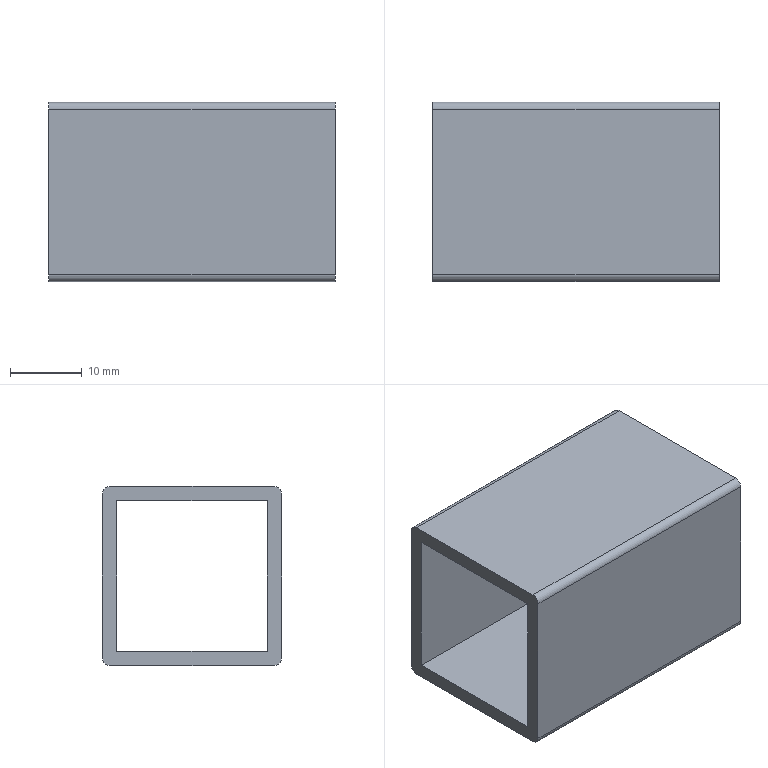Part | SolidWorks | features BreakCorner 1, FlatPattern 1, SMBaseFlange 1, SheetMetal 1 | 1 solid | 14 faces | box 40 x 25 x 25 mm | volume 7326 mm3 | plane 10 | cylinder 4 | commonest cylinder face diameters 2 x4
STEP:
#1=CARTESIAN_POINT('',(-40.,11.5,12.5));
#2=VERTEX_POINT('',#1);
#3=CARTESIAN_POINT('',(-40.,-11.5,12.5));
#4=VERTEX_POINT('',#3);
#5=CARTESIAN_POINT('',(-40.,12.5,12.5));
#6=DIRECTION('',(0.,-1.,0.));
#7=VECTOR('',#6,1000.);
#8=LINE('',#5,#7);
#9=EDGE_CURVE('',#2,#4,#8,.T.);
#10=ORIENTED_EDGE('',*,*,#9,.T.);
#11=CARTESIAN_POINT('',(0.,-11.5,12.5));
#12=VERTEX_POINT('',#11);
#13=CARTESIAN_POINT('',(-40.,-11.5,12.5));
#14=DIRECTION('',(1.,0.,0.));
#15=VECTOR('',#14,1000.);
#16=LINE('',#13,#15);
#17=EDGE_CURVE('',#4,#12,#16,.T.);
#18=ORIENTED_EDGE('',*,*,#17,.T.);
#19=CARTESIAN_POINT('',(0.,11.5,12.5));
#20=VERTEX_POINT('',#19);
#21=CARTESIAN_POINT('',(0.,12.5,12.5));
#22=DIRECTION('',(0.,-1.,0.));
#23=VECTOR('',#22,1000.);
#24=LINE('',#21,#23);
#25=EDGE_CURVE('',#20,#12,#24,.T.);
#26=ORIENTED_EDGE('',*,*,#25,.F.);
#27=CARTESIAN_POINT('',(-40.,11.5,12.5));
#28=DIRECTION('',(-1.,0.,0.));
#29=VECTOR('',#28,1000.);
#30=LINE('',#27,#29);
#31=EDGE_CURVE('',#20,#2,#30,.T.);
#32=ORIENTED_EDGE('',*,*,#31,.T.);
#33=EDGE_LOOP('',(#10,#18,#26,#32));
#34=FACE_OUTER_BOUND('',#33,.T.);
#35=CARTESIAN_POINT('',(-40.,12.5,12.5));
#36=DIRECTION('',(0.,0.,1.));
#37=DIRECTION('',(0.,-1.,0.));
#38=AXIS2_PLACEMENT_3D('',#35,#36,#37);
#39=PLANE('',#38);
#40=ADVANCED_FACE('',(#34),#39,.T.);
#41=CARTESIAN_POINT('',(0.,12.5,-11.5));
#42=VERTEX_POINT('',#41);
#43=CARTESIAN_POINT('',(0.,12.5,11.5));
#44=VERTEX_POINT('',#43);
#45=CARTESIAN_POINT('',(0.,12.5,12.5));
#46=DIRECTION('',(0.,0.,1.));
#47=VECTOR('',#46,1000.);
#48=LINE('',#45,#47);
#49=EDGE_CURVE('',#42,#44,#48,.T.);
#50=ORIENTED_EDGE('',*,*,#49,.F.);
#51=CARTESIAN_POINT('',(-40.,12.5,-11.5));
#52=VERTEX_POINT('',#51);
#53=CARTESIAN_POINT('',(-40.,12.5,-11.5));
#54=DIRECTION('',(-1.,0.,0.));
#55=VECTOR('',#54,1000.);
#56=LINE('',#53,#55);
#57=EDGE_CURVE('',#42,#52,#56,.T.);
#58=ORIENTED_EDGE('',*,*,#57,.T.);
#59=CARTESIAN_POINT('',(-40.,12.5,11.5));
#60=VERTEX_POINT('',#59);
#61=CARTESIAN_POINT('',(-40.,12.5,12.5));
#62=DIRECTION('',(0.,0.,1.));
#63=VECTOR('',#62,1000.);
#64=LINE('',#61,#63);
#65=EDGE_CURVE('',#52,#60,#64,.T.);
#66=ORIENTED_EDGE('',*,*,#65,.T.);
#67=CARTESIAN_POINT('',(-40.,12.5,11.5));
#68=DIRECTION('',(1.,0.,0.));
#69=VECTOR('',#68,1000.);
#70=LINE('',#67,#69);
#71=EDGE_CURVE('',#60,#44,#70,.T.);
#72=ORIENTED_EDGE('',*,*,#71,.T.);
#73=EDGE_LOOP('',(#50,#58,#66,#72));
#74=FACE_OUTER_BOUND('',#73,.T.);
#75=CARTESIAN_POINT('',(-40.,12.5,12.5));
#76=DIRECTION('',(0.,1.,0.));
#77=DIRECTION('',(0.,0.,1.));
#78=AXIS2_PLACEMENT_3D('',#75,#76,#77);
#79=PLANE('',#78);
#80=ADVANCED_FACE('',(#74),#79,.T.);
#81=CARTESIAN_POINT('',(0.,-11.5,-12.5));
#82=VERTEX_POINT('',#81);
#83=CARTESIAN_POINT('',(0.,11.5,-12.5));
#84=VERTEX_POINT('',#83);
#85=CARTESIAN_POINT('',(0.,12.5,-12.5));
#86=DIRECTION('',(0.,1.,0.));
#87=VECTOR('',#86,1000.);
#88=LINE('',#85,#87);
#89=EDGE_CURVE('',#82,#84,#88,.T.);
#90=ORIENTED_EDGE('',*,*,#89,.F.);
#91=CARTESIAN_POINT('',(-40.,-11.5,-12.5));
#92=VERTEX_POINT('',#91);
#93=CARTESIAN_POINT('',(-40.,-11.5,-12.5));
#94=DIRECTION('',(-1.,0.,0.));
#95=VECTOR('',#94,1000.);
#96=LINE('',#93,#95);
#97=EDGE_CURVE('',#82,#92,#96,.T.);
#98=ORIENTED_EDGE('',*,*,#97,.T.);
#99=CARTESIAN_POINT('',(-40.,11.5,-12.5));
#100=VERTEX_POINT('',#99);
#101=CARTESIAN_POINT('',(-40.,12.5,-12.5));
#102=DIRECTION('',(0.,1.,0.));
#103=VECTOR('',#102,1000.);
#104=LINE('',#101,#103);
#105=EDGE_CURVE('',#92,#100,#104,.T.);
#106=ORIENTED_EDGE('',*,*,#105,.T.);
#107=CARTESIAN_POINT('',(-40.,11.5,-12.5));
#108=DIRECTION('',(1.,0.,0.));
#109=VECTOR('',#108,1000.);
#110=LINE('',#107,#109);
#111=EDGE_CURVE('',#100,#84,#110,.T.);
#112=ORIENTED_EDGE('',*,*,#111,.T.);
#113=EDGE_LOOP('',(#90,#98,#106,#112));
#114=FACE_OUTER_BOUND('',#113,.T.);
#115=CARTESIAN_POINT('',(-40.,12.5,-12.5));
#116=DIRECTION('',(0.,0.,-1.));
#117=DIRECTION('',(0.,1.,0.));
#118=AXIS2_PLACEMENT_3D('',#115,#116,#117);
#119=PLANE('',#118);
#120=ADVANCED_FACE('',(#114),#119,.T.);
#121=CARTESIAN_POINT('',(-40.,-12.5,11.5));
#122=VERTEX_POINT('',#121);
#123=CARTESIAN_POINT('',(-40.,-12.5,-11.5));
#124=VERTEX_POINT('',#123);
#125=CARTESIAN_POINT('',(-40.,-12.5,12.5));
#126=DIRECTION('',(0.,0.,-1.));
#127=VECTOR('',#126,1000.);
#128=LINE('',#125,#127);
#129=EDGE_CURVE('',#122,#124,#128,.T.);
#130=ORIENTED_EDGE('',*,*,#129,.T.);
#131=CARTESIAN_POINT('',(0.,-12.5,-11.5));
#132=VERTEX_POINT('',#131);
#133=CARTESIAN_POINT('',(-40.,-12.5,-11.5));
#134=DIRECTION('',(1.,0.,0.));
#135=VECTOR('',#134,1000.);
#136=LINE('',#133,#135);
#137=EDGE_CURVE('',#124,#132,#136,.T.);
#138=ORIENTED_EDGE('',*,*,#137,.T.);
#139=CARTESIAN_POINT('',(0.,-12.5,11.5));
#140=VERTEX_POINT('',#139);
#141=CARTESIAN_POINT('',(0.,-12.5,12.5));
#142=DIRECTION('',(0.,0.,-1.));
#143=VECTOR('',#142,1000.);
#144=LINE('',#141,#143);
#145=EDGE_CURVE('',#140,#132,#144,.T.);
#146=ORIENTED_EDGE('',*,*,#145,.F.);
#147=CARTESIAN_POINT('',(-40.,-12.5,11.5));
#148=DIRECTION('',(-1.,0.,0.));
#149=VECTOR('',#148,1000.);
#150=LINE('',#147,#149);
#151=EDGE_CURVE('',#140,#122,#150,.T.);
#152=ORIENTED_EDGE('',*,*,#151,.T.);
#153=EDGE_LOOP('',(#130,#138,#146,#152));
#154=FACE_OUTER_BOUND('',#153,.T.);
#155=CARTESIAN_POINT('',(-40.,-12.5,12.5));
#156=DIRECTION('',(0.,-1.,0.));
#157=DIRECTION('',(0.,0.,-1.));
#158=AXIS2_PLACEMENT_3D('',#155,#156,#157);
#159=PLANE('',#158);
#160=ADVANCED_FACE('',(#154),#159,.T.);
#161=CARTESIAN_POINT('',(-40.,-10.5,10.5));
#162=VERTEX_POINT('',#161);
#163=CARTESIAN_POINT('',(-40.,-10.5,-10.5));
#164=VERTEX_POINT('',#163);
#165=CARTESIAN_POINT('',(-40.,-10.5,10.5));
#166=DIRECTION('',(0.,0.,-1.));
#167=VECTOR('',#166,1000.);
#168=LINE('',#165,#167);
#169=EDGE_CURVE('',#162,#164,#168,.T.);
#170=ORIENTED_EDGE('',*,*,#169,.T.);
#171=CARTESIAN_POINT('',(-40.,10.5,-10.5));
#172=VERTEX_POINT('',#171);
#173=CARTESIAN_POINT('',(-40.,10.5,-10.5));
#174=DIRECTION('',(0.,1.,0.));
#175=VECTOR('',#174,1000.);
#176=LINE('',#173,#175);
#177=EDGE_CURVE('',#164,#172,#176,.T.);
#178=ORIENTED_EDGE('',*,*,#177,.T.);
#179=CARTESIAN_POINT('',(-40.,10.5,10.5));
#180=VERTEX_POINT('',#179);
#181=CARTESIAN_POINT('',(-40.,10.5,10.5));
#182=DIRECTION('',(0.,0.,1.));
#183=VECTOR('',#182,1000.);
#184=LINE('',#181,#183);
#185=EDGE_CURVE('',#172,#180,#184,.T.);
#186=ORIENTED_EDGE('',*,*,#185,.T.);
#187=CARTESIAN_POINT('',(-40.,10.5,10.5));
#188=DIRECTION('',(0.,-1.,0.));
#189=VECTOR('',#188,1000.);
#190=LINE('',#187,#189);
#191=EDGE_CURVE('',#180,#162,#190,.T.);
#192=ORIENTED_EDGE('',*,*,#191,.T.);
#193=EDGE_LOOP('',(#170,#178,#186,#192));
#194=FACE_BOUND('',#193,.T.);
#195=ORIENTED_EDGE('',*,*,#105,.F.);
#196=CARTESIAN_POINT('',(-40.,-11.5,-11.5));
#197=DIRECTION('',(-1.,0.,0.));
#198=DIRECTION('',(0.,0.,-1.));
#199=AXIS2_PLACEMENT_3D('',#196,#197,#198);
#200=CIRCLE('',#199,1.);
#201=EDGE_CURVE('',#92,#124,#200,.T.);
#202=ORIENTED_EDGE('',*,*,#201,.T.);
#203=ORIENTED_EDGE('',*,*,#129,.F.);
#204=CARTESIAN_POINT('',(-40.,-11.5,11.5));
#205=DIRECTION('',(-1.,0.,0.));
#206=DIRECTION('',(0.,0.,-1.));
#207=AXIS2_PLACEMENT_3D('',#204,#205,#206);
#208=CIRCLE('',#207,1.);
#209=EDGE_CURVE('',#122,#4,#208,.T.);
#210=ORIENTED_EDGE('',*,*,#209,.T.);
#211=ORIENTED_EDGE('',*,*,#9,.F.);
#212=CARTESIAN_POINT('',(-40.,11.5,11.5));
#213=DIRECTION('',(-1.,0.,0.));
#214=DIRECTION('',(0.,0.,-1.));
#215=AXIS2_PLACEMENT_3D('',#212,#213,#214);
#216=CIRCLE('',#215,1.);
#217=EDGE_CURVE('',#2,#60,#216,.T.);
#218=ORIENTED_EDGE('',*,*,#217,.T.);
#219=ORIENTED_EDGE('',*,*,#65,.F.);
#220=CARTESIAN_POINT('',(-40.,11.5,-11.5));
#221=DIRECTION('',(-1.,0.,0.));
#222=DIRECTION('',(0.,0.,-1.));
#223=AXIS2_PLACEMENT_3D('',#220,#221,#222);
#224=CIRCLE('',#223,1.);
#225=EDGE_CURVE('',#52,#100,#224,.T.);
#226=ORIENTED_EDGE('',*,*,#225,.T.);
#227=EDGE_LOOP('',(#195,#202,#203,#210,#211,#218,#219,#226));
#228=FACE_OUTER_BOUND('',#227,.T.);
#229=CARTESIAN_POINT('',(-40.,0.,0.));
#230=DIRECTION('',(1.,0.,0.));
#231=DIRECTION('',(0.,0.,-1.));
#232=AXIS2_PLACEMENT_3D('',#229,#230,#231);
#233=PLANE('',#232);
#234=ADVANCED_FACE('',(#194,#228),#233,.F.);
#235=CARTESIAN_POINT('',(0.,-10.5,-10.5));
#236=VERTEX_POINT('',#235);
#237=CARTESIAN_POINT('',(0.,10.5,-10.5));
#238=VERTEX_POINT('',#237);
#239=CARTESIAN_POINT('',(0.,10.5,-10.5));
#240=DIRECTION('',(0.,1.,0.));
#241=VECTOR('',#240,1000.);
#242=LINE('',#239,#241);
#243=EDGE_CURVE('',#236,#238,#242,.T.);
#244=ORIENTED_EDGE('',*,*,#243,.F.);
#245=CARTESIAN_POINT('',(0.,-10.5,10.5));
#246=VERTEX_POINT('',#245);
#247=CARTESIAN_POINT('',(0.,-10.5,10.5));
#248=DIRECTION('',(0.,0.,-1.));
#249=VECTOR('',#248,1000.);
#250=LINE('',#247,#249);
#251=EDGE_CURVE('',#246,#236,#250,.T.);
#252=ORIENTED_EDGE('',*,*,#251,.F.);
#253=CARTESIAN_POINT('',(0.,10.5,10.5));
#254=VERTEX_POINT('',#253);
#255=CARTESIAN_POINT('',(0.,10.5,10.5));
#256=DIRECTION('',(0.,-1.,0.));
#257=VECTOR('',#256,1000.);
#258=LINE('',#255,#257);
#259=EDGE_CURVE('',#254,#246,#258,.T.);
#260=ORIENTED_EDGE('',*,*,#259,.F.);
#261=CARTESIAN_POINT('',(0.,10.5,10.5));
#262=DIRECTION('',(0.,0.,1.));
#263=VECTOR('',#262,1000.);
#264=LINE('',#261,#263);
#265=EDGE_CURVE('',#238,#254,#264,.T.);
#266=ORIENTED_EDGE('',*,*,#265,.F.);
#267=EDGE_LOOP('',(#244,#252,#260,#266));
#268=FACE_BOUND('',#267,.T.);
#269=ORIENTED_EDGE('',*,*,#145,.T.);
#270=CARTESIAN_POINT('',(0.,-11.5,-11.5));
#271=DIRECTION('',(1.,0.,0.));
#272=DIRECTION('',(0.,0.,-1.));
#273=AXIS2_PLACEMENT_3D('',#270,#271,#272);
#274=CIRCLE('',#273,1.);
#275=EDGE_CURVE('',#132,#82,#274,.T.);
#276=ORIENTED_EDGE('',*,*,#275,.T.);
#277=ORIENTED_EDGE('',*,*,#89,.T.);
#278=CARTESIAN_POINT('',(0.,11.5,-11.5));
#279=DIRECTION('',(1.,0.,0.));
#280=DIRECTION('',(0.,0.,-1.));
#281=AXIS2_PLACEMENT_3D('',#278,#279,#280);
#282=CIRCLE('',#281,1.);
#283=EDGE_CURVE('',#84,#42,#282,.T.);
#284=ORIENTED_EDGE('',*,*,#283,.T.);
#285=ORIENTED_EDGE('',*,*,#49,.T.);
#286=CARTESIAN_POINT('',(0.,11.5,11.5));
#287=DIRECTION('',(1.,0.,0.));
#288=DIRECTION('',(0.,0.,-1.));
#289=AXIS2_PLACEMENT_3D('',#286,#287,#288);
#290=CIRCLE('',#289,1.);
#291=EDGE_CURVE('',#44,#20,#290,.T.);
#292=ORIENTED_EDGE('',*,*,#291,.T.);
#293=ORIENTED_EDGE('',*,*,#25,.T.);
#294=CARTESIAN_POINT('',(0.,-11.5,11.5));
#295=DIRECTION('',(1.,0.,0.));
#296=DIRECTION('',(0.,0.,-1.));
#297=AXIS2_PLACEMENT_3D('',#294,#295,#296);
#298=CIRCLE('',#297,1.);
#299=EDGE_CURVE('',#12,#140,#298,.T.);
#300=ORIENTED_EDGE('',*,*,#299,.T.);
#301=EDGE_LOOP('',(#269,#276,#277,#284,#285,#292,#293,#300));
#302=FACE_OUTER_BOUND('',#301,.T.);
#303=CARTESIAN_POINT('',(0.,0.,0.));
#304=DIRECTION('',(1.,0.,0.));
#305=DIRECTION('',(0.,0.,-1.));
#306=AXIS2_PLACEMENT_3D('',#303,#304,#305);
#307=PLANE('',#306);
#308=ADVANCED_FACE('',(#268,#302),#307,.T.);
#309=ORIENTED_EDGE('',*,*,#243,.T.);
#310=CARTESIAN_POINT('',(-40.,10.5,-10.5));
#311=DIRECTION('',(1.,0.,0.));
#312=VECTOR('',#311,1000.);
#313=LINE('',#310,#312);
#314=EDGE_CURVE('',#172,#238,#313,.T.);
#315=ORIENTED_EDGE('',*,*,#314,.F.);
#316=ORIENTED_EDGE('',*,*,#177,.F.);
#317=CARTESIAN_POINT('',(-40.,-10.5,-10.5));
#318=DIRECTION('',(1.,0.,0.));
#319=VECTOR('',#318,1000.);
#320=LINE('',#317,#319);
#321=EDGE_CURVE('',#164,#236,#320,.T.);
#322=ORIENTED_EDGE('',*,*,#321,.T.);
#323=EDGE_LOOP('',(#309,#315,#316,#322));
#324=FACE_OUTER_BOUND('',#323,.T.);
#325=CARTESIAN_POINT('',(-40.,10.5,-10.5));
#326=DIRECTION('',(0.,0.,-1.));
#327=DIRECTION('',(0.,1.,0.));
#328=AXIS2_PLACEMENT_3D('',#325,#326,#327);
#329=PLANE('',#328);
#330=ADVANCED_FACE('',(#324),#329,.F.);
#331=ORIENTED_EDGE('',*,*,#251,.T.);
#332=ORIENTED_EDGE('',*,*,#321,.F.);
#333=ORIENTED_EDGE('',*,*,#169,.F.);
#334=CARTESIAN_POINT('',(-40.,-10.5,10.5));
#335=DIRECTION('',(1.,0.,0.));
#336=VECTOR('',#335,1000.);
#337=LINE('',#334,#336);
#338=EDGE_CURVE('',#162,#246,#337,.T.);
#339=ORIENTED_EDGE('',*,*,#338,.T.);
#340=EDGE_LOOP('',(#331,#332,#333,#339));
#341=FACE_OUTER_BOUND('',#340,.T.);
#342=CARTESIAN_POINT('',(-40.,-10.5,10.5));
#343=DIRECTION('',(0.,-1.,0.));
#344=DIRECTION('',(0.,0.,-1.));
#345=AXIS2_PLACEMENT_3D('',#342,#343,#344);
#346=PLANE('',#345);
#347=ADVANCED_FACE('',(#341),#346,.F.);
#348=ORIENTED_EDGE('',*,*,#259,.T.);
#349=ORIENTED_EDGE('',*,*,#338,.F.);
#350=ORIENTED_EDGE('',*,*,#191,.F.);
#351=CARTESIAN_POINT('',(-40.,10.5,10.5));
#352=DIRECTION('',(1.,0.,0.));
#353=VECTOR('',#352,1000.);
#354=LINE('',#351,#353);
#355=EDGE_CURVE('',#180,#254,#354,.T.);
#356=ORIENTED_EDGE('',*,*,#355,.T.);
#357=EDGE_LOOP('',(#348,#349,#350,#356));
#358=FACE_OUTER_BOUND('',#357,.T.);
#359=CARTESIAN_POINT('',(-40.,10.5,10.5));
#360=DIRECTION('',(0.,0.,1.));
#361=DIRECTION('',(1.,0.,0.));
#362=AXIS2_PLACEMENT_3D('',#359,#360,#361);
#363=PLANE('',#362);
#364=ADVANCED_FACE('',(#358),#363,.F.);
#365=ORIENTED_EDGE('',*,*,#265,.T.);
#366=ORIENTED_EDGE('',*,*,#355,.F.);
#367=ORIENTED_EDGE('',*,*,#185,.F.);
#368=ORIENTED_EDGE('',*,*,#314,.T.);
#369=EDGE_LOOP('',(#365,#366,#367,#368));
#370=FACE_OUTER_BOUND('',#369,.T.);
#371=CARTESIAN_POINT('',(-40.,10.5,10.5));
#372=DIRECTION('',(0.,1.,0.));
#373=DIRECTION('',(0.,0.,1.));
#374=AXIS2_PLACEMENT_3D('',#371,#372,#373);
#375=PLANE('',#374);
#376=ADVANCED_FACE('',(#370),#375,.F.);
#377=ORIENTED_EDGE('',*,*,#201,.F.);
#378=ORIENTED_EDGE('',*,*,#97,.F.);
#379=ORIENTED_EDGE('',*,*,#275,.F.);
#380=ORIENTED_EDGE('',*,*,#137,.F.);
#381=EDGE_LOOP('',(#377,#378,#379,#380));
#382=FACE_OUTER_BOUND('',#381,.T.);
#383=CARTESIAN_POINT('',(-40.,-11.5,-11.5));
#384=DIRECTION('',(1.,0.,0.));
#385=DIRECTION('',(0.,0.,-1.));
#386=AXIS2_PLACEMENT_3D('',#383,#384,#385);
#387=CYLINDRICAL_SURFACE('',#386,1.);
#388=ADVANCED_FACE('',(#382),#387,.T.);
#389=ORIENTED_EDGE('',*,*,#209,.F.);
#390=ORIENTED_EDGE('',*,*,#151,.F.);
#391=ORIENTED_EDGE('',*,*,#299,.F.);
#392=ORIENTED_EDGE('',*,*,#17,.F.);
#393=EDGE_LOOP('',(#389,#390,#391,#392));
#394=FACE_OUTER_BOUND('',#393,.T.);
#395=CARTESIAN_POINT('',(-40.,-11.5,11.5));
#396=DIRECTION('',(1.,0.,0.));
#397=DIRECTION('',(0.,0.,-1.));
#398=AXIS2_PLACEMENT_3D('',#395,#396,#397);
#399=CYLINDRICAL_SURFACE('',#398,1.);
#400=ADVANCED_FACE('',(#394),#399,.T.);
#401=ORIENTED_EDGE('',*,*,#225,.F.);
#402=ORIENTED_EDGE('',*,*,#57,.F.);
#403=ORIENTED_EDGE('',*,*,#283,.F.);
#404=ORIENTED_EDGE('',*,*,#111,.F.);
#405=EDGE_LOOP('',(#401,#402,#403,#404));
#406=FACE_OUTER_BOUND('',#405,.T.);
#407=CARTESIAN_POINT('',(-40.,11.5,-11.5));
#408=DIRECTION('',(1.,0.,0.));
#409=DIRECTION('',(0.,0.,-1.));
#410=AXIS2_PLACEMENT_3D('',#407,#408,#409);
#411=CYLINDRICAL_SURFACE('',#410,1.);
#412=ADVANCED_FACE('',(#406),#411,.T.);
#413=ORIENTED_EDGE('',*,*,#217,.F.);
#414=ORIENTED_EDGE('',*,*,#31,.F.);
#415=ORIENTED_EDGE('',*,*,#291,.F.);
#416=ORIENTED_EDGE('',*,*,#71,.F.);
#417=EDGE_LOOP('',(#413,#414,#415,#416));
#418=FACE_OUTER_BOUND('',#417,.T.);
#419=CARTESIAN_POINT('',(-40.,11.5,11.5));
#420=DIRECTION('',(1.,0.,0.));
#421=DIRECTION('',(0.,0.,-1.));
#422=AXIS2_PLACEMENT_3D('',#419,#420,#421);
#423=CYLINDRICAL_SURFACE('',#422,1.);
#424=ADVANCED_FACE('',(#418),#423,.T.);
#425=CLOSED_SHELL('',(#40,#80,#120,#160,#234,#308,#330,#347,#364,#376,#388,#400,#412,#424));
#426=MANIFOLD_SOLID_BREP('',#425);
#427=CARTESIAN_POINT('',(0.,0.,0.));
#428=DIRECTION('',(0.,0.,1.));
#429=DIRECTION('',(1.,0.,0.));
#430=AXIS2_PLACEMENT_3D('',#427,#428,#429);
#431=(LENGTH_UNIT()NAMED_UNIT(*)SI_UNIT(.MILLI.,.METRE.));
#432=UNCERTAINTY_MEASURE_WITH_UNIT(LENGTH_MEASURE(0.00001),#431,'','');
#433=(NAMED_UNIT(*)PLANE_ANGLE_UNIT()SI_UNIT($,.RADIAN.));
#434=(NAMED_UNIT(*)SI_UNIT($,.STERADIAN.)SOLID_ANGLE_UNIT());
#435=(GEOMETRIC_REPRESENTATION_CONTEXT(3)GLOBAL_UNCERTAINTY_ASSIGNED_CONTEXT((#432))GLOBAL_UNIT_ASSIGNED_CONTEXT((#431,#433,#434))REPRESENTATION_CONTEXT('',''));
#436=ADVANCED_BREP_SHAPE_REPRESENTATION('',(#426,#430),#435);